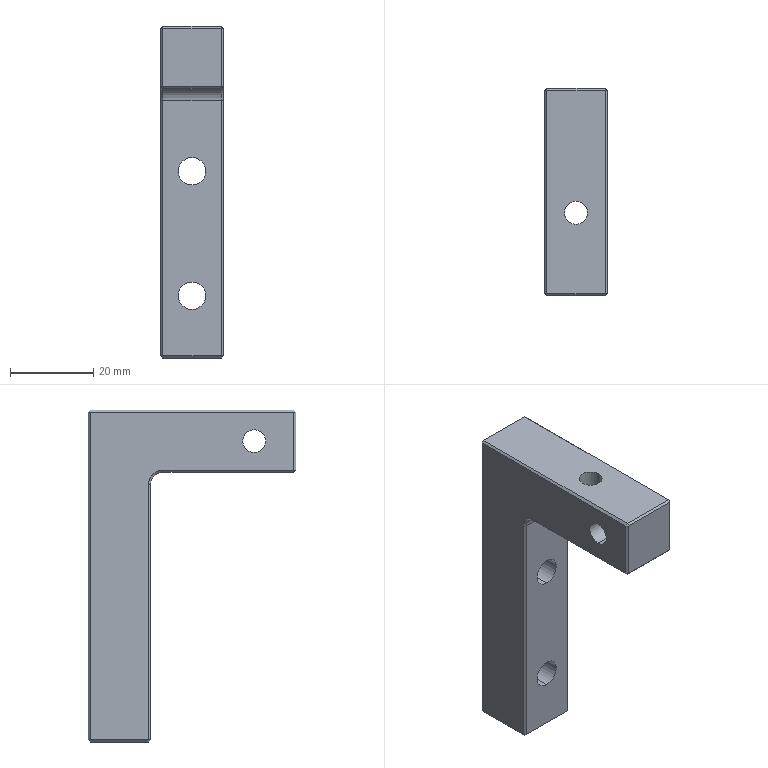Part | SolidWorks | features HoleWzd 3, Chamfer 1, Extrusion 1, Fillet 1, ICE 1, LPattern 1 | 1 solid | 46 faces | box 15 x 50 x 80 mm | volume 24092 mm3 | plane 35 | cylinder 9 | cone 2 | commonest cylinder face diameters 5.5 x4 6.6 x4 6 x1
STEP:
#1=CARTESIAN_POINT('',(97.5,-49.,204.8));
#2=VERTEX_POINT('',#1);
#3=CARTESIAN_POINT('',(97.5,-49.,198.2));
#4=VERTEX_POINT('',#3);
#5=CARTESIAN_POINT('',(97.5,-49.,201.5));
#6=DIRECTION('',(0.,-1.,0.));
#7=DIRECTION('',(0.,0.,-1.));
#8=AXIS2_PLACEMENT_3D('',#5,#6,#7);
#9=CIRCLE('',#8,3.3);
#10=EDGE_CURVE('',#2,#4,#9,.T.);
#11=ORIENTED_EDGE('',*,*,#10,.F.);
#12=CARTESIAN_POINT('',(97.5,-64.,204.8));
#13=VERTEX_POINT('',#12);
#14=CARTESIAN_POINT('',(97.5,-64.,204.8));
#15=DIRECTION('',(0.,-1.,0.));
#16=VECTOR('',#15,1000.);
#17=LINE('',#14,#16);
#18=EDGE_CURVE('',#2,#13,#17,.T.);
#19=ORIENTED_EDGE('',*,*,#18,.T.);
#20=CARTESIAN_POINT('',(97.5,-64.,198.2));
#21=VERTEX_POINT('',#20);
#22=CARTESIAN_POINT('',(97.5,-64.,201.5));
#23=DIRECTION('',(0.,-1.,0.));
#24=DIRECTION('',(0.,0.,-1.));
#25=AXIS2_PLACEMENT_3D('',#22,#23,#24);
#26=CIRCLE('',#25,3.3);
#27=EDGE_CURVE('',#13,#21,#26,.T.);
#28=ORIENTED_EDGE('',*,*,#27,.T.);
#29=CARTESIAN_POINT('',(97.5,-64.,198.2));
#30=DIRECTION('',(0.,-1.,0.));
#31=VECTOR('',#30,1000.);
#32=LINE('',#29,#31);
#33=EDGE_CURVE('',#4,#21,#32,.T.);
#34=ORIENTED_EDGE('',*,*,#33,.F.);
#35=EDGE_LOOP('',(#11,#19,#28,#34));
#36=FACE_OUTER_BOUND('',#35,.T.);
#37=CARTESIAN_POINT('',(97.5,-64.,201.5));
#38=DIRECTION('',(0.,-1.,0.));
#39=DIRECTION('',(0.,0.,-1.));
#40=AXIS2_PLACEMENT_3D('',#37,#38,#39);
#41=CYLINDRICAL_SURFACE('',#40,3.3);
#42=ADVANCED_FACE('',(#36),#41,.F.);
#43=CARTESIAN_POINT('',(105.,-89.,226.25));
#44=VERTEX_POINT('',#43);
#45=CARTESIAN_POINT('',(105.,-89.,231.75));
#46=VERTEX_POINT('',#45);
#47=CARTESIAN_POINT('',(105.,-89.,229.));
#48=DIRECTION('',(-1.,0.,0.));
#49=DIRECTION('',(0.,0.,1.));
#50=AXIS2_PLACEMENT_3D('',#47,#48,#49);
#51=CIRCLE('',#50,2.75);
#52=EDGE_CURVE('',#44,#46,#51,.T.);
#53=ORIENTED_EDGE('',*,*,#52,.F.);
#54=CARTESIAN_POINT('',(90.,-89.,226.25));
#55=VERTEX_POINT('',#54);
#56=CARTESIAN_POINT('',(90.,-89.,226.25));
#57=DIRECTION('',(-1.,0.,0.));
#58=VECTOR('',#57,1000.);
#59=LINE('',#56,#58);
#60=EDGE_CURVE('',#44,#55,#59,.T.);
#61=ORIENTED_EDGE('',*,*,#60,.T.);
#62=CARTESIAN_POINT('',(90.,-89.,231.75));
#63=VERTEX_POINT('',#62);
#64=CARTESIAN_POINT('',(90.,-89.,229.));
#65=DIRECTION('',(-1.,0.,0.));
#66=DIRECTION('',(0.,0.,1.));
#67=AXIS2_PLACEMENT_3D('',#64,#65,#66);
#68=CIRCLE('',#67,2.75);
#69=EDGE_CURVE('',#55,#63,#68,.T.);
#70=ORIENTED_EDGE('',*,*,#69,.T.);
#71=CARTESIAN_POINT('',(90.,-89.,231.75));
#72=DIRECTION('',(-1.,0.,0.));
#73=VECTOR('',#72,1000.);
#74=LINE('',#71,#73);
#75=EDGE_CURVE('',#46,#63,#74,.T.);
#76=ORIENTED_EDGE('',*,*,#75,.F.);
#77=EDGE_LOOP('',(#53,#61,#70,#76));
#78=FACE_OUTER_BOUND('',#77,.T.);
#79=CARTESIAN_POINT('',(90.,-89.,229.));
#80=DIRECTION('',(-1.,0.,0.));
#81=DIRECTION('',(0.,0.,1.));
#82=AXIS2_PLACEMENT_3D('',#79,#80,#81);
#83=CYLINDRICAL_SURFACE('',#82,2.75);
#84=ADVANCED_FACE('',(#78),#83,.F.);
#85=CARTESIAN_POINT('',(100.25,-79.,236.5));
#86=VERTEX_POINT('',#85);
#87=CARTESIAN_POINT('',(94.75,-79.,236.5));
#88=VERTEX_POINT('',#87);
#89=CARTESIAN_POINT('',(97.5,-79.,236.5));
#90=DIRECTION('',(0.,0.,-1.));
#91=DIRECTION('',(-1.,0.,0.));
#92=AXIS2_PLACEMENT_3D('',#89,#90,#91);
#93=CIRCLE('',#92,2.75);
#94=EDGE_CURVE('',#86,#88,#93,.T.);
#95=ORIENTED_EDGE('',*,*,#94,.F.);
#96=CARTESIAN_POINT('',(100.25,-79.,221.5));
#97=VERTEX_POINT('',#96);
#98=CARTESIAN_POINT('',(100.25,-79.,221.5));
#99=DIRECTION('',(0.,0.,-1.));
#100=VECTOR('',#99,1000.);
#101=LINE('',#98,#100);
#102=EDGE_CURVE('',#86,#97,#101,.T.);
#103=ORIENTED_EDGE('',*,*,#102,.T.);
#104=CARTESIAN_POINT('',(94.75,-79.,221.5));
#105=VERTEX_POINT('',#104);
#106=CARTESIAN_POINT('',(97.5,-79.,221.5));
#107=DIRECTION('',(0.,0.,-1.));
#108=DIRECTION('',(-1.,0.,0.));
#109=AXIS2_PLACEMENT_3D('',#106,#107,#108);
#110=CIRCLE('',#109,2.75);
#111=EDGE_CURVE('',#97,#105,#110,.T.);
#112=ORIENTED_EDGE('',*,*,#111,.T.);
#113=CARTESIAN_POINT('',(94.75,-79.,221.5));
#114=DIRECTION('',(0.,0.,-1.));
#115=VECTOR('',#114,1000.);
#116=LINE('',#113,#115);
#117=EDGE_CURVE('',#88,#105,#116,.T.);
#118=ORIENTED_EDGE('',*,*,#117,.F.);
#119=EDGE_LOOP('',(#95,#103,#112,#118));
#120=FACE_OUTER_BOUND('',#119,.T.);
#121=CARTESIAN_POINT('',(97.5,-79.,221.5));
#122=DIRECTION('',(0.,0.,-1.));
#123=DIRECTION('',(-1.,0.,0.));
#124=AXIS2_PLACEMENT_3D('',#121,#122,#123);
#125=CYLINDRICAL_SURFACE('',#124,2.75);
#126=ADVANCED_FACE('',(#120),#125,.F.);
#127=CARTESIAN_POINT('',(97.5,-49.,174.8));
#128=VERTEX_POINT('',#127);
#129=CARTESIAN_POINT('',(97.5,-49.,168.2));
#130=VERTEX_POINT('',#129);
#131=CARTESIAN_POINT('',(97.5,-49.,171.5));
#132=DIRECTION('',(0.,-1.,0.));
#133=DIRECTION('',(0.,0.,-1.));
#134=AXIS2_PLACEMENT_3D('',#131,#132,#133);
#135=CIRCLE('',#134,3.3);
#136=EDGE_CURVE('',#128,#130,#135,.T.);
#137=ORIENTED_EDGE('',*,*,#136,.F.);
#138=CARTESIAN_POINT('',(97.5,-64.,174.8));
#139=VERTEX_POINT('',#138);
#140=CARTESIAN_POINT('',(97.5,-64.,174.8));
#141=DIRECTION('',(0.,-1.,0.));
#142=VECTOR('',#141,1000.);
#143=LINE('',#140,#142);
#144=EDGE_CURVE('',#128,#139,#143,.T.);
#145=ORIENTED_EDGE('',*,*,#144,.T.);
#146=CARTESIAN_POINT('',(97.5,-64.,168.2));
#147=VERTEX_POINT('',#146);
#148=CARTESIAN_POINT('',(97.5,-64.,171.5));
#149=DIRECTION('',(0.,-1.,0.));
#150=DIRECTION('',(0.,0.,-1.));
#151=AXIS2_PLACEMENT_3D('',#148,#149,#150);
#152=CIRCLE('',#151,3.3);
#153=EDGE_CURVE('',#139,#147,#152,.T.);
#154=ORIENTED_EDGE('',*,*,#153,.T.);
#155=CARTESIAN_POINT('',(97.5,-64.,168.2));
#156=DIRECTION('',(0.,-1.,0.));
#157=VECTOR('',#156,1000.);
#158=LINE('',#155,#157);
#159=EDGE_CURVE('',#130,#147,#158,.T.);
#160=ORIENTED_EDGE('',*,*,#159,.F.);
#161=EDGE_LOOP('',(#137,#145,#154,#160));
#162=FACE_OUTER_BOUND('',#161,.T.);
#163=CARTESIAN_POINT('',(97.5,-64.,171.5));
#164=DIRECTION('',(0.,-1.,0.));
#165=DIRECTION('',(0.,0.,-1.));
#166=AXIS2_PLACEMENT_3D('',#163,#164,#165);
#167=CYLINDRICAL_SURFACE('',#166,3.3);
#168=ADVANCED_FACE('',(#162),#167,.F.);
#169=CARTESIAN_POINT('',(97.5,-64.,201.5));
#170=DIRECTION('',(0.,-1.,0.));
#171=DIRECTION('',(0.,0.,-1.));
#172=AXIS2_PLACEMENT_3D('',#169,#170,#171);
#173=CIRCLE('',#172,3.3);
#174=EDGE_CURVE('',#21,#13,#173,.T.);
#175=ORIENTED_EDGE('',*,*,#174,.F.);
#176=ORIENTED_EDGE('',*,*,#27,.F.);
#177=EDGE_LOOP('',(#175,#176));
#178=FACE_BOUND('',#177,.T.);
#179=CARTESIAN_POINT('',(104.5,-64.,218.5));
#180=VERTEX_POINT('',#179);
#181=CARTESIAN_POINT('',(90.5,-64.,218.5));
#182=VERTEX_POINT('',#181);
#183=CARTESIAN_POINT('',(90.,-64.,218.5));
#184=DIRECTION('',(-1.,0.,0.));
#185=VECTOR('',#184,1000.);
#186=LINE('',#183,#185);
#187=EDGE_CURVE('',#180,#182,#186,.T.);
#188=ORIENTED_EDGE('',*,*,#187,.T.);
#189=CARTESIAN_POINT('',(90.5,-64.,157.));
#190=VERTEX_POINT('',#189);
#191=CARTESIAN_POINT('',(90.5,-64.,156.5));
#192=DIRECTION('',(0.,0.,-1.));
#193=VECTOR('',#192,1000.);
#194=LINE('',#191,#193);
#195=EDGE_CURVE('',#182,#190,#194,.T.);
#196=ORIENTED_EDGE('',*,*,#195,.T.);
#197=CARTESIAN_POINT('',(104.5,-64.,157.));
#198=VERTEX_POINT('',#197);
#199=CARTESIAN_POINT('',(105.,-64.,157.));
#200=DIRECTION('',(1.,0.,0.));
#201=VECTOR('',#200,1000.);
#202=LINE('',#199,#201);
#203=EDGE_CURVE('',#190,#198,#202,.T.);
#204=ORIENTED_EDGE('',*,*,#203,.T.);
#205=CARTESIAN_POINT('',(104.5,-64.,156.5));
#206=DIRECTION('',(0.,0.,1.));
#207=VECTOR('',#206,1000.);
#208=LINE('',#205,#207);
#209=EDGE_CURVE('',#198,#180,#208,.T.);
#210=ORIENTED_EDGE('',*,*,#209,.T.);
#211=EDGE_LOOP('',(#188,#196,#204,#210));
#212=FACE_OUTER_BOUND('',#211,.T.);
#213=CARTESIAN_POINT('',(97.5,-64.,171.5));
#214=DIRECTION('',(0.,-1.,0.));
#215=DIRECTION('',(0.,0.,-1.));
#216=AXIS2_PLACEMENT_3D('',#213,#214,#215);
#217=CIRCLE('',#216,3.3);
#218=EDGE_CURVE('',#147,#139,#217,.T.);
#219=ORIENTED_EDGE('',*,*,#218,.F.);
#220=ORIENTED_EDGE('',*,*,#153,.F.);
#221=EDGE_LOOP('',(#219,#220));
#222=FACE_BOUND('',#221,.T.);
#223=CARTESIAN_POINT('',(105.,-64.,156.5));
#224=DIRECTION('',(0.,1.,0.));
#225=DIRECTION('',(0.,0.,1.));
#226=AXIS2_PLACEMENT_3D('',#223,#224,#225);
#227=PLANE('',#226);
#228=ADVANCED_FACE('',(#178,#212,#222),#227,.F.);
#229=CARTESIAN_POINT('',(90.,-89.,229.));
#230=DIRECTION('',(-1.,0.,0.));
#231=DIRECTION('',(0.,0.,1.));
#232=AXIS2_PLACEMENT_3D('',#229,#230,#231);
#233=CIRCLE('',#232,2.75);
#234=EDGE_CURVE('',#63,#55,#233,.T.);
#235=ORIENTED_EDGE('',*,*,#234,.F.);
#236=ORIENTED_EDGE('',*,*,#69,.F.);
#237=EDGE_LOOP('',(#235,#236));
#238=FACE_BOUND('',#237,.T.);
#239=CARTESIAN_POINT('',(90.,-49.5,157.));
#240=VERTEX_POINT('',#239);
#241=CARTESIAN_POINT('',(90.,-63.5,157.));
#242=VERTEX_POINT('',#241);
#243=CARTESIAN_POINT('',(90.,-64.,157.));
#244=DIRECTION('',(0.,-1.,0.));
#245=VECTOR('',#244,1000.);
#246=LINE('',#243,#245);
#247=EDGE_CURVE('',#240,#242,#246,.T.);
#248=ORIENTED_EDGE('',*,*,#247,.T.);
#249=CARTESIAN_POINT('',(90.,-63.5,218.5));
#250=VERTEX_POINT('',#249);
#251=CARTESIAN_POINT('',(90.,-63.5,156.5));
#252=DIRECTION('',(0.,0.,1.));
#253=VECTOR('',#252,1000.);
#254=LINE('',#251,#253);
#255=EDGE_CURVE('',#242,#250,#254,.T.);
#256=ORIENTED_EDGE('',*,*,#255,.T.);
#257=CARTESIAN_POINT('',(90.,-67.,222.));
#258=VERTEX_POINT('',#257);
#259=CARTESIAN_POINT('',(90.,-67.,218.5));
#260=DIRECTION('',(1.,0.,0.));
#261=DIRECTION('',(0.,0.,-1.));
#262=AXIS2_PLACEMENT_3D('',#259,#260,#261);
#263=CIRCLE('',#262,3.5);
#264=EDGE_CURVE('',#250,#258,#263,.T.);
#265=ORIENTED_EDGE('',*,*,#264,.T.);
#266=CARTESIAN_POINT('',(90.,-98.5,222.));
#267=VERTEX_POINT('',#266);
#268=CARTESIAN_POINT('',(90.,-49.,222.));
#269=DIRECTION('',(0.,-1.,0.));
#270=VECTOR('',#269,1000.);
#271=LINE('',#268,#270);
#272=EDGE_CURVE('',#258,#267,#271,.T.);
#273=ORIENTED_EDGE('',*,*,#272,.T.);
#274=CARTESIAN_POINT('',(90.,-98.5,236.));
#275=VERTEX_POINT('',#274);
#276=CARTESIAN_POINT('',(90.,-98.5,156.5));
#277=DIRECTION('',(0.,0.,1.));
#278=VECTOR('',#277,1000.);
#279=LINE('',#276,#278);
#280=EDGE_CURVE('',#267,#275,#279,.T.);
#281=ORIENTED_EDGE('',*,*,#280,.T.);
#282=CARTESIAN_POINT('',(90.,-49.5,236.));
#283=VERTEX_POINT('',#282);
#284=CARTESIAN_POINT('',(90.,-49.,236.));
#285=DIRECTION('',(0.,1.,0.));
#286=VECTOR('',#285,1000.);
#287=LINE('',#284,#286);
#288=EDGE_CURVE('',#275,#283,#287,.T.);
#289=ORIENTED_EDGE('',*,*,#288,.T.);
#290=CARTESIAN_POINT('',(90.,-49.5,156.5));
#291=DIRECTION('',(0.,0.,-1.));
#292=VECTOR('',#291,1000.);
#293=LINE('',#290,#292);
#294=EDGE_CURVE('',#283,#240,#293,.T.);
#295=ORIENTED_EDGE('',*,*,#294,.T.);
#296=EDGE_LOOP('',(#248,#256,#265,#273,#281,#289,#295));
#297=FACE_OUTER_BOUND('',#296,.T.);
#298=CARTESIAN_POINT('',(90.,-49.,156.5));
#299=DIRECTION('',(1.,0.,0.));
#300=DIRECTION('',(0.,0.,-1.));
#301=AXIS2_PLACEMENT_3D('',#298,#299,#300);
#302=PLANE('',#301);
#303=ADVANCED_FACE('',(#238,#297),#302,.F.);
#304=CARTESIAN_POINT('',(97.5,-49.,201.5));
#305=DIRECTION('',(0.,-1.,0.));
#306=DIRECTION('',(0.,0.,-1.));
#307=AXIS2_PLACEMENT_3D('',#304,#305,#306);
#308=CIRCLE('',#307,3.3);
#309=EDGE_CURVE('',#4,#2,#308,.T.);
#310=ORIENTED_EDGE('',*,*,#309,.T.);
#311=ORIENTED_EDGE('',*,*,#10,.T.);
#312=EDGE_LOOP('',(#310,#311));
#313=FACE_BOUND('',#312,.T.);
#314=CARTESIAN_POINT('',(90.5,-49.,236.));
#315=VERTEX_POINT('',#314);
#316=CARTESIAN_POINT('',(104.5,-49.,236.));
#317=VERTEX_POINT('',#316);
#318=CARTESIAN_POINT('',(90.,-49.,236.));
#319=DIRECTION('',(1.,0.,0.));
#320=VECTOR('',#319,1000.);
#321=LINE('',#318,#320);
#322=EDGE_CURVE('',#315,#317,#321,.T.);
#323=ORIENTED_EDGE('',*,*,#322,.T.);
#324=CARTESIAN_POINT('',(104.5,-49.,157.));
#325=VERTEX_POINT('',#324);
#326=CARTESIAN_POINT('',(104.5,-49.,156.5));
#327=DIRECTION('',(0.,0.,-1.));
#328=VECTOR('',#327,1000.);
#329=LINE('',#326,#328);
#330=EDGE_CURVE('',#317,#325,#329,.T.);
#331=ORIENTED_EDGE('',*,*,#330,.T.);
#332=CARTESIAN_POINT('',(90.5,-49.,157.));
#333=VERTEX_POINT('',#332);
#334=CARTESIAN_POINT('',(90.,-49.,157.));
#335=DIRECTION('',(-1.,0.,0.));
#336=VECTOR('',#335,1000.);
#337=LINE('',#334,#336);
#338=EDGE_CURVE('',#325,#333,#337,.T.);
#339=ORIENTED_EDGE('',*,*,#338,.T.);
#340=CARTESIAN_POINT('',(90.5,-49.,156.5));
#341=DIRECTION('',(0.,0.,1.));
#342=VECTOR('',#341,1000.);
#343=LINE('',#340,#342);
#344=EDGE_CURVE('',#333,#315,#343,.T.);
#345=ORIENTED_EDGE('',*,*,#344,.T.);
#346=EDGE_LOOP('',(#323,#331,#339,#345));
#347=FACE_OUTER_BOUND('',#346,.T.);
#348=CARTESIAN_POINT('',(97.5,-49.,171.5));
#349=DIRECTION('',(0.,-1.,0.));
#350=DIRECTION('',(0.,0.,-1.));
#351=AXIS2_PLACEMENT_3D('',#348,#349,#350);
#352=CIRCLE('',#351,3.3);
#353=EDGE_CURVE('',#130,#128,#352,.T.);
#354=ORIENTED_EDGE('',*,*,#353,.T.);
#355=ORIENTED_EDGE('',*,*,#136,.T.);
#356=EDGE_LOOP('',(#354,#355));
#357=FACE_BOUND('',#356,.T.);
#358=CARTESIAN_POINT('',(90.,-49.,156.5));
#359=DIRECTION('',(0.,-1.,0.));
#360=DIRECTION('',(1.,0.,0.));
#361=AXIS2_PLACEMENT_3D('',#358,#359,#360);
#362=PLANE('',#361);
#363=ADVANCED_FACE('',(#313,#347,#357),#362,.F.);
#364=CARTESIAN_POINT('',(105.,-89.,229.));
#365=DIRECTION('',(-1.,0.,0.));
#366=DIRECTION('',(0.,0.,1.));
#367=AXIS2_PLACEMENT_3D('',#364,#365,#366);
#368=CIRCLE('',#367,2.75);
#369=EDGE_CURVE('',#46,#44,#368,.T.);
#370=ORIENTED_EDGE('',*,*,#369,.T.);
#371=ORIENTED_EDGE('',*,*,#52,.T.);
#372=EDGE_LOOP('',(#370,#371));
#373=FACE_BOUND('',#372,.T.);
#374=CARTESIAN_POINT('',(105.,-63.5,157.));
#375=VERTEX_POINT('',#374);
#376=CARTESIAN_POINT('',(105.,-49.5,157.));
#377=VERTEX_POINT('',#376);
#378=CARTESIAN_POINT('',(105.,-49.,157.));
#379=DIRECTION('',(0.,1.,0.));
#380=VECTOR('',#379,1000.);
#381=LINE('',#378,#380);
#382=EDGE_CURVE('',#375,#377,#381,.T.);
#383=ORIENTED_EDGE('',*,*,#382,.T.);
#384=CARTESIAN_POINT('',(105.,-49.5,236.));
#385=VERTEX_POINT('',#384);
#386=CARTESIAN_POINT('',(105.,-49.5,156.5));
#387=DIRECTION('',(0.,0.,1.));
#388=VECTOR('',#387,1000.);
#389=LINE('',#386,#388);
#390=EDGE_CURVE('',#377,#385,#389,.T.);
#391=ORIENTED_EDGE('',*,*,#390,.T.);
#392=CARTESIAN_POINT('',(105.,-98.5,236.));
#393=VERTEX_POINT('',#392);
#394=CARTESIAN_POINT('',(105.,-49.,236.));
#395=DIRECTION('',(0.,-1.,0.));
#396=VECTOR('',#395,1000.);
#397=LINE('',#394,#396);
#398=EDGE_CURVE('',#385,#393,#397,.T.);
#399=ORIENTED_EDGE('',*,*,#398,.T.);
#400=CARTESIAN_POINT('',(105.,-98.5,222.));
#401=VERTEX_POINT('',#400);
#402=CARTESIAN_POINT('',(105.,-98.5,156.5));
#403=DIRECTION('',(0.,0.,-1.));
#404=VECTOR('',#403,1000.);
#405=LINE('',#402,#404);
#406=EDGE_CURVE('',#393,#401,#405,.T.);
#407=ORIENTED_EDGE('',*,*,#406,.T.);
#408=CARTESIAN_POINT('',(105.,-67.,222.));
#409=VERTEX_POINT('',#408);
#410=CARTESIAN_POINT('',(105.,-49.,222.));
#411=DIRECTION('',(0.,1.,0.));
#412=VECTOR('',#411,1000.);
#413=LINE('',#410,#412);
#414=EDGE_CURVE('',#401,#409,#413,.T.);
#415=ORIENTED_EDGE('',*,*,#414,.T.);
#416=CARTESIAN_POINT('',(105.,-63.5,218.5));
#417=VERTEX_POINT('',#416);
#418=CARTESIAN_POINT('',(105.,-67.,218.5));
#419=DIRECTION('',(-1.,0.,0.));
#420=DIRECTION('',(0.,-1.,0.));
#421=AXIS2_PLACEMENT_3D('',#418,#419,#420);
#422=CIRCLE('',#421,3.5);
#423=EDGE_CURVE('',#409,#417,#422,.T.);
#424=ORIENTED_EDGE('',*,*,#423,.T.);
#425=CARTESIAN_POINT('',(105.,-63.5,156.5));
#426=DIRECTION('',(0.,0.,-1.));
#427=VECTOR('',#426,1000.);
#428=LINE('',#425,#427);
#429=EDGE_CURVE('',#417,#375,#428,.T.);
#430=ORIENTED_EDGE('',*,*,#429,.T.);
#431=EDGE_LOOP('',(#383,#391,#399,#407,#415,#424,#430));
#432=FACE_OUTER_BOUND('',#431,.T.);
#433=CARTESIAN_POINT('',(105.,-49.,156.5));
#434=DIRECTION('',(-1.,0.,0.));
#435=DIRECTION('',(0.,-1.,0.));
#436=AXIS2_PLACEMENT_3D('',#433,#434,#435);
#437=PLANE('',#436);
#438=ADVANCED_FACE('',(#373,#432),#437,.F.);
#439=CARTESIAN_POINT('',(90.5,-49.5,156.5));
#440=VERTEX_POINT('',#439);
#441=CARTESIAN_POINT('',(104.5,-49.5,156.5));
#442=VERTEX_POINT('',#441);
#443=CARTESIAN_POINT('',(105.,-49.5,156.5));
#444=DIRECTION('',(1.,0.,0.));
#445=VECTOR('',#444,1000.);
#446=LINE('',#443,#445);
#447=EDGE_CURVE('',#440,#442,#446,.T.);
#448=ORIENTED_EDGE('',*,*,#447,.T.);
#449=CARTESIAN_POINT('',(104.5,-63.5,156.5));
#450=VERTEX_POINT('',#449);
#451=CARTESIAN_POINT('',(104.5,-64.,156.5));
#452=DIRECTION('',(0.,-1.,0.));
#453=VECTOR('',#452,1000.);
#454=LINE('',#451,#453);
#455=EDGE_CURVE('',#442,#450,#454,.T.);
#456=ORIENTED_EDGE('',*,*,#455,.T.);
#457=CARTESIAN_POINT('',(90.5,-63.5,156.5));
#458=VERTEX_POINT('',#457);
#459=CARTESIAN_POINT('',(90.,-63.5,156.5));
#460=DIRECTION('',(-1.,0.,0.));
#461=VECTOR('',#460,1000.);
#462=LINE('',#459,#461);
#463=EDGE_CURVE('',#450,#458,#462,.T.);
#464=ORIENTED_EDGE('',*,*,#463,.T.);
#465=CARTESIAN_POINT('',(90.5,-49.,156.5));
#466=DIRECTION('',(0.,1.,0.));
#467=VECTOR('',#466,1000.);
#468=LINE('',#465,#467);
#469=EDGE_CURVE('',#458,#440,#468,.T.);
#470=ORIENTED_EDGE('',*,*,#469,.T.);
#471=EDGE_LOOP('',(#448,#456,#464,#470));
#472=FACE_OUTER_BOUND('',#471,.T.);
#473=CARTESIAN_POINT('',(90.,-64.,156.5));
#474=DIRECTION('',(0.,0.,-1.));
#475=DIRECTION('',(-1.,0.,0.));
#476=AXIS2_PLACEMENT_3D('',#473,#474,#475);
#477=PLANE('',#476);
#478=ADVANCED_FACE('',(#472),#477,.T.);
#479=CARTESIAN_POINT('',(97.5,-79.,236.5));
#480=DIRECTION('',(0.,0.,-1.));
#481=DIRECTION('',(-1.,0.,0.));
#482=AXIS2_PLACEMENT_3D('',#479,#480,#481);
#483=CIRCLE('',#482,2.75);
#484=EDGE_CURVE('',#88,#86,#483,.T.);
#485=ORIENTED_EDGE('',*,*,#484,.T.);
#486=ORIENTED_EDGE('',*,*,#94,.T.);
#487=EDGE_LOOP('',(#485,#486));
#488=FACE_BOUND('',#487,.T.);
#489=CARTESIAN_POINT('',(90.5,-98.5,236.5));
#490=VERTEX_POINT('',#489);
#491=CARTESIAN_POINT('',(104.5,-98.5,236.5));
#492=VERTEX_POINT('',#491);
#493=CARTESIAN_POINT('',(90.,-98.5,236.5));
#494=DIRECTION('',(1.,0.,0.));
#495=VECTOR('',#494,1000.);
#496=LINE('',#493,#495);
#497=EDGE_CURVE('',#490,#492,#496,.T.);
#498=ORIENTED_EDGE('',*,*,#497,.T.);
#499=CARTESIAN_POINT('',(104.5,-49.5,236.5));
#500=VERTEX_POINT('',#499);
#501=CARTESIAN_POINT('',(104.5,-64.,236.5));
#502=DIRECTION('',(0.,1.,0.));
#503=VECTOR('',#502,1000.);
#504=LINE('',#501,#503);
#505=EDGE_CURVE('',#492,#500,#504,.T.);
#506=ORIENTED_EDGE('',*,*,#505,.T.);
#507=CARTESIAN_POINT('',(90.5,-49.5,236.5));
#508=VERTEX_POINT('',#507);
#509=CARTESIAN_POINT('',(90.,-49.5,236.5));
#510=DIRECTION('',(-1.,0.,0.));
#511=VECTOR('',#510,1000.);
#512=LINE('',#509,#511);
#513=EDGE_CURVE('',#500,#508,#512,.T.);
#514=ORIENTED_EDGE('',*,*,#513,.T.);
#515=CARTESIAN_POINT('',(90.5,-64.,236.5));
#516=DIRECTION('',(0.,-1.,0.));
#517=VECTOR('',#516,1000.);
#518=LINE('',#515,#517);
#519=EDGE_CURVE('',#508,#490,#518,.T.);
#520=ORIENTED_EDGE('',*,*,#519,.T.);
#521=EDGE_LOOP('',(#498,#506,#514,#520));
#522=FACE_OUTER_BOUND('',#521,.T.);
#523=CARTESIAN_POINT('',(90.,-64.,236.5));
#524=DIRECTION('',(0.,0.,-1.));
#525=DIRECTION('',(-1.,0.,0.));
#526=AXIS2_PLACEMENT_3D('',#523,#524,#525);
#527=PLANE('',#526);
#528=ADVANCED_FACE('',(#488,#522),#527,.F.);
#529=ORIENTED_EDGE('',*,*,#144,.F.);
#530=ORIENTED_EDGE('',*,*,#353,.F.);
#531=ORIENTED_EDGE('',*,*,#159,.T.);
#532=ORIENTED_EDGE('',*,*,#218,.T.);
#533=EDGE_LOOP('',(#529,#530,#531,#532));
#534=FACE_OUTER_BOUND('',#533,.T.);
#535=CARTESIAN_POINT('',(97.5,-64.,171.5));
#536=DIRECTION('',(0.,-1.,0.));
#537=DIRECTION('',(0.,0.,-1.));
#538=AXIS2_PLACEMENT_3D('',#535,#536,#537);
#539=CYLINDRICAL_SURFACE('',#538,3.3);
#540=ADVANCED_FACE('',(#534),#539,.F.);
#541=CARTESIAN_POINT('',(97.5,-79.,221.5));
#542=DIRECTION('',(0.,0.,-1.));
#543=DIRECTION('',(-1.,0.,0.));
#544=AXIS2_PLACEMENT_3D('',#541,#542,#543);
#545=CIRCLE('',#544,2.75);
#546=EDGE_CURVE('',#105,#97,#545,.T.);
#547=ORIENTED_EDGE('',*,*,#546,.F.);
#548=ORIENTED_EDGE('',*,*,#111,.F.);
#549=EDGE_LOOP('',(#547,#548));
#550=FACE_BOUND('',#549,.T.);
#551=CARTESIAN_POINT('',(90.5,-67.,221.5));
#552=VERTEX_POINT('',#551);
#553=CARTESIAN_POINT('',(104.5,-67.,221.5));
#554=VERTEX_POINT('',#553);
#555=CARTESIAN_POINT('',(105.,-67.,221.5));
#556=DIRECTION('',(1.,0.,0.));
#557=VECTOR('',#556,1000.);
#558=LINE('',#555,#557);
#559=EDGE_CURVE('',#552,#554,#558,.T.);
#560=ORIENTED_EDGE('',*,*,#559,.T.);
#561=CARTESIAN_POINT('',(104.5,-98.5,221.5));
#562=VERTEX_POINT('',#561);
#563=CARTESIAN_POINT('',(104.5,-99.,221.5));
#564=DIRECTION('',(0.,-1.,0.));
#565=VECTOR('',#564,1000.);
#566=LINE('',#563,#565);
#567=EDGE_CURVE('',#554,#562,#566,.T.);
#568=ORIENTED_EDGE('',*,*,#567,.T.);
#569=CARTESIAN_POINT('',(90.5,-98.5,221.5));
#570=VERTEX_POINT('',#569);
#571=CARTESIAN_POINT('',(90.,-98.5,221.5));
#572=DIRECTION('',(-1.,0.,0.));
#573=VECTOR('',#572,1000.);
#574=LINE('',#571,#573);
#575=EDGE_CURVE('',#562,#570,#574,.T.);
#576=ORIENTED_EDGE('',*,*,#575,.T.);
#577=CARTESIAN_POINT('',(90.5,-99.,221.5));
#578=DIRECTION('',(0.,1.,0.));
#579=VECTOR('',#578,1000.);
#580=LINE('',#577,#579);
#581=EDGE_CURVE('',#570,#552,#580,.T.);
#582=ORIENTED_EDGE('',*,*,#581,.T.);
#583=EDGE_LOOP('',(#560,#568,#576,#582));
#584=FACE_OUTER_BOUND('',#583,.T.);
#585=CARTESIAN_POINT('',(90.,-99.,221.5));
#586=DIRECTION('',(0.,0.,1.));
#587=DIRECTION('',(1.,0.,0.));
#588=AXIS2_PLACEMENT_3D('',#585,#586,#587);
#589=PLANE('',#588);
#590=ADVANCED_FACE('',(#550,#584),#589,.F.);
#591=CARTESIAN_POINT('',(90.5,-99.,222.));
#592=VERTEX_POINT('',#591);
#593=CARTESIAN_POINT('',(104.5,-99.,222.));
#594=VERTEX_POINT('',#593);
#595=CARTESIAN_POINT('',(90.,-99.,222.));
#596=DIRECTION('',(1.,0.,0.));
#597=VECTOR('',#596,1000.);
#598=LINE('',#595,#597);
#599=EDGE_CURVE('',#592,#594,#598,.T.);
#600=ORIENTED_EDGE('',*,*,#599,.T.);
#601=CARTESIAN_POINT('',(104.5,-99.,236.));
#602=VERTEX_POINT('',#601);
#603=CARTESIAN_POINT('',(104.5,-99.,236.5));
#604=DIRECTION('',(0.,0.,1.));
#605=VECTOR('',#604,1000.);
#606=LINE('',#603,#605);
#607=EDGE_CURVE('',#594,#602,#606,.T.);
#608=ORIENTED_EDGE('',*,*,#607,.T.);
#609=CARTESIAN_POINT('',(90.5,-99.,236.));
#610=VERTEX_POINT('',#609);
#611=CARTESIAN_POINT('',(90.,-99.,236.));
#612=DIRECTION('',(-1.,0.,0.));
#613=VECTOR('',#612,1000.);
#614=LINE('',#611,#613);
#615=EDGE_CURVE('',#602,#610,#614,.T.);
#616=ORIENTED_EDGE('',*,*,#615,.T.);
#617=CARTESIAN_POINT('',(90.5,-99.,236.5));
#618=DIRECTION('',(0.,0.,-1.));
#619=VECTOR('',#618,1000.);
#620=LINE('',#617,#619);
#621=EDGE_CURVE('',#610,#592,#620,.T.);
#622=ORIENTED_EDGE('',*,*,#621,.T.);
#623=EDGE_LOOP('',(#600,#608,#616,#622));
#624=FACE_OUTER_BOUND('',#623,.T.);
#625=CARTESIAN_POINT('',(90.,-99.,236.5));
#626=DIRECTION('',(0.,1.,0.));
#627=DIRECTION('',(0.,0.,1.));
#628=AXIS2_PLACEMENT_3D('',#625,#626,#627);
#629=PLANE('',#628);
#630=ADVANCED_FACE('',(#624),#629,.F.);
#631=ORIENTED_EDGE('',*,*,#559,.F.);
#632=CARTESIAN_POINT('',(90.5,-67.,218.5));
#633=DIRECTION('',(-1.,0.,0.));
#634=DIRECTION('',(0.,0.,-1.));
#635=AXIS2_PLACEMENT_3D('',#632,#633,#634);
#636=CIRCLE('',#635,3.);
#637=EDGE_CURVE('',#552,#182,#636,.T.);
#638=ORIENTED_EDGE('',*,*,#637,.T.);
#639=ORIENTED_EDGE('',*,*,#187,.F.);
#640=CARTESIAN_POINT('',(104.5,-67.,218.5));
#641=DIRECTION('',(1.,0.,0.));
#642=DIRECTION('',(0.,0.,1.));
#643=AXIS2_PLACEMENT_3D('',#640,#641,#642);
#644=CIRCLE('',#643,3.);
#645=EDGE_CURVE('',#180,#554,#644,.T.);
#646=ORIENTED_EDGE('',*,*,#645,.T.);
#647=EDGE_LOOP('',(#631,#638,#639,#646));
#648=FACE_OUTER_BOUND('',#647,.T.);
#649=CARTESIAN_POINT('',(90.,-67.,218.5));
#650=DIRECTION('',(-1.,0.,0.));
#651=DIRECTION('',(0.,0.,1.));
#652=AXIS2_PLACEMENT_3D('',#649,#650,#651);
#653=CYLINDRICAL_SURFACE('',#652,3.);
#654=ADVANCED_FACE('',(#648),#653,.F.);
#655=CARTESIAN_POINT('',(105.,-49.5,236.));
#656=DIRECTION('',(0.7071,0.,-0.7071));
#657=VECTOR('',#656,1000.);
#658=LINE('',#655,#657);
#659=EDGE_CURVE('',#500,#385,#658,.T.);
#660=ORIENTED_EDGE('',*,*,#659,.F.);
#661=ORIENTED_EDGE('',*,*,#505,.F.);
#662=CARTESIAN_POINT('',(104.75,-98.5,236.25));
#663=DIRECTION('',(-0.7071,0.,0.7071));
#664=VECTOR('',#663,1000.);
#665=LINE('',#662,#664);
#666=EDGE_CURVE('',#393,#492,#665,.T.);
#667=ORIENTED_EDGE('',*,*,#666,.F.);
#668=ORIENTED_EDGE('',*,*,#398,.F.);
#669=EDGE_LOOP('',(#660,#661,#667,#668));
#670=FACE_OUTER_BOUND('',#669,.T.);
#671=CARTESIAN_POINT('',(105.,-49.,236.));
#672=DIRECTION('',(-0.7071,0.,-0.7071));
#673=DIRECTION('',(-0.7071,0.,0.7071));
#674=AXIS2_PLACEMENT_3D('',#671,#672,#673);
#675=PLANE('',#674);
#676=ADVANCED_FACE('',(#670),#675,.F.);
#677=CARTESIAN_POINT('',(104.5,-49.25,236.25));
#678=DIRECTION('',(0.,0.7071,-0.7071));
#679=VECTOR('',#678,1000.);
#680=LINE('',#677,#679);
#681=EDGE_CURVE('',#500,#317,#680,.T.);
#682=ORIENTED_EDGE('',*,*,#681,.F.);
#683=ORIENTED_EDGE('',*,*,#659,.T.);
#684=CARTESIAN_POINT('',(105.,-49.5,236.));
#685=DIRECTION('',(0.7071,-0.7071,0.));
#686=VECTOR('',#685,1000.);
#687=LINE('',#684,#686);
#688=EDGE_CURVE('',#317,#385,#687,.T.);
#689=ORIENTED_EDGE('',*,*,#688,.F.);
#690=EDGE_LOOP('',(#682,#683,#689));
#691=FACE_OUTER_BOUND('',#690,.T.);
#692=CARTESIAN_POINT('',(105.,-49.5,236.));
#693=DIRECTION('',(0.5774,0.5774,0.5774));
#694=DIRECTION('',(-0.7071,0.7071,0.));
#695=AXIS2_PLACEMENT_3D('',#692,#693,#694);
#696=PLANE('',#695);
#697=ADVANCED_FACE('',(#691),#696,.T.);
#698=CARTESIAN_POINT('',(104.5,-99.,236.));
#699=DIRECTION('',(-0.7071,-0.7071,0.));
#700=VECTOR('',#699,1000.);
#701=LINE('',#698,#700);
#702=EDGE_CURVE('',#393,#602,#701,.T.);
#703=ORIENTED_EDGE('',*,*,#702,.F.);
#704=ORIENTED_EDGE('',*,*,#666,.T.);
#705=CARTESIAN_POINT('',(104.5,-99.,236.));
#706=DIRECTION('',(0.,0.7071,0.7071));
#707=VECTOR('',#706,1000.);
#708=LINE('',#705,#707);
#709=EDGE_CURVE('',#602,#492,#708,.T.);
#710=ORIENTED_EDGE('',*,*,#709,.F.);
#711=EDGE_LOOP('',(#703,#704,#710));
#712=FACE_OUTER_BOUND('',#711,.T.);
#713=CARTESIAN_POINT('',(104.5,-99.,236.));
#714=DIRECTION('',(0.5774,-0.5774,0.5774));
#715=DIRECTION('',(0.7071,0.7071,0.));
#716=AXIS2_PLACEMENT_3D('',#713,#714,#715);
#717=PLANE('',#716);
#718=ADVANCED_FACE('',(#712),#717,.T.);
#719=ORIENTED_EDGE('',*,*,#688,.T.);
#720=ORIENTED_EDGE('',*,*,#390,.F.);
#721=CARTESIAN_POINT('',(104.5,-49.,157.));
#722=DIRECTION('',(0.7071,-0.7071,0.));
#723=VECTOR('',#722,1000.);
#724=LINE('',#721,#723);
#725=EDGE_CURVE('',#325,#377,#724,.T.);
#726=ORIENTED_EDGE('',*,*,#725,.F.);
#727=ORIENTED_EDGE('',*,*,#330,.F.);
#728=EDGE_LOOP('',(#719,#720,#726,#727));
#729=FACE_OUTER_BOUND('',#728,.T.);
#730=CARTESIAN_POINT('',(105.,-49.5,156.5));
#731=DIRECTION('',(-0.7071,-0.7071,0.));
#732=DIRECTION('',(0.7071,-0.7071,0.));
#733=AXIS2_PLACEMENT_3D('',#730,#731,#732);
#734=PLANE('',#733);
#735=ADVANCED_FACE('',(#729),#734,.F.);
#736=ORIENTED_EDGE('',*,*,#681,.T.);
#737=ORIENTED_EDGE('',*,*,#322,.F.);
#738=CARTESIAN_POINT('',(90.5,-49.,236.));
#739=DIRECTION('',(0.,0.7071,-0.7071));
#740=VECTOR('',#739,1000.);
#741=LINE('',#738,#740);
#742=EDGE_CURVE('',#508,#315,#741,.T.);
#743=ORIENTED_EDGE('',*,*,#742,.F.);
#744=ORIENTED_EDGE('',*,*,#513,.F.);
#745=EDGE_LOOP('',(#736,#737,#743,#744));
#746=FACE_OUTER_BOUND('',#745,.T.);
#747=CARTESIAN_POINT('',(90.,-49.,236.));
#748=DIRECTION('',(0.,-0.7071,-0.7071));
#749=DIRECTION('',(0.,0.7071,-0.7071));
#750=AXIS2_PLACEMENT_3D('',#747,#748,#749);
#751=PLANE('',#750);
#752=ADVANCED_FACE('',(#746),#751,.F.);
#753=CARTESIAN_POINT('',(90.,-98.5,236.));
#754=DIRECTION('',(-0.7071,0.,-0.7071));
#755=VECTOR('',#754,1000.);
#756=LINE('',#753,#755);
#757=EDGE_CURVE('',#490,#275,#756,.T.);
#758=ORIENTED_EDGE('',*,*,#757,.F.);
#759=ORIENTED_EDGE('',*,*,#519,.F.);
#760=CARTESIAN_POINT('',(90.25,-49.5,236.25));
#761=DIRECTION('',(0.7071,0.,0.7071));
#762=VECTOR('',#761,1000.);
#763=LINE('',#760,#762);
#764=EDGE_CURVE('',#283,#508,#763,.T.);
#765=ORIENTED_EDGE('',*,*,#764,.F.);
#766=ORIENTED_EDGE('',*,*,#288,.F.);
#767=EDGE_LOOP('',(#758,#759,#765,#766));
#768=FACE_OUTER_BOUND('',#767,.T.);
#769=CARTESIAN_POINT('',(90.,-49.,236.));
#770=DIRECTION('',(0.7071,0.,-0.7071));
#771=DIRECTION('',(-0.7071,0.,-0.7071));
#772=AXIS2_PLACEMENT_3D('',#769,#770,#771);
#773=PLANE('',#772);
#774=ADVANCED_FACE('',(#768),#773,.F.);
#775=ORIENTED_EDGE('',*,*,#709,.T.);
#776=ORIENTED_EDGE('',*,*,#497,.F.);
#777=CARTESIAN_POINT('',(90.5,-98.75,236.25));
#778=DIRECTION('',(0.,0.7071,0.7071));
#779=VECTOR('',#778,1000.);
#780=LINE('',#777,#779);
#781=EDGE_CURVE('',#610,#490,#780,.T.);
#782=ORIENTED_EDGE('',*,*,#781,.F.);
#783=ORIENTED_EDGE('',*,*,#615,.F.);
#784=EDGE_LOOP('',(#775,#776,#782,#783));
#785=FACE_OUTER_BOUND('',#784,.T.);
#786=CARTESIAN_POINT('',(90.,-99.,236.));
#787=DIRECTION('',(0.,0.7071,-0.7071));
#788=DIRECTION('',(0.,0.7071,0.7071));
#789=AXIS2_PLACEMENT_3D('',#786,#787,#788);
#790=PLANE('',#789);
#791=ADVANCED_FACE('',(#785),#790,.F.);
#792=ORIENTED_EDGE('',*,*,#702,.T.);
#793=ORIENTED_EDGE('',*,*,#607,.F.);
#794=CARTESIAN_POINT('',(104.75,-98.75,222.));
#795=DIRECTION('',(-0.7071,-0.7071,0.));
#796=VECTOR('',#795,1000.);
#797=LINE('',#794,#796);
#798=EDGE_CURVE('',#401,#594,#797,.T.);
#799=ORIENTED_EDGE('',*,*,#798,.F.);
#800=ORIENTED_EDGE('',*,*,#406,.F.);
#801=EDGE_LOOP('',(#792,#793,#799,#800));
#802=FACE_OUTER_BOUND('',#801,.T.);
#803=CARTESIAN_POINT('',(104.5,-99.,236.5));
#804=DIRECTION('',(-0.7071,0.7071,0.));
#805=DIRECTION('',(-0.7071,-0.7071,0.));
#806=AXIS2_PLACEMENT_3D('',#803,#804,#805);
#807=PLANE('',#806);
#808=ADVANCED_FACE('',(#802),#807,.F.);
#809=CARTESIAN_POINT('',(104.5,-98.5,221.5));
#810=DIRECTION('',(0.7071,0.,0.7071));
#811=VECTOR('',#810,1000.);
#812=LINE('',#809,#811);
#813=EDGE_CURVE('',#562,#401,#812,.T.);
#814=ORIENTED_EDGE('',*,*,#813,.F.);
#815=ORIENTED_EDGE('',*,*,#567,.F.);
#816=CARTESIAN_POINT('',(105.,-67.,222.));
#817=DIRECTION('',(-0.7071,0.,-0.7071));
#818=VECTOR('',#817,1000.);
#819=LINE('',#816,#818);
#820=EDGE_CURVE('',#409,#554,#819,.T.);
#821=ORIENTED_EDGE('',*,*,#820,.F.);
#822=ORIENTED_EDGE('',*,*,#414,.F.);
#823=EDGE_LOOP('',(#814,#815,#821,#822));
#824=FACE_OUTER_BOUND('',#823,.T.);
#825=CARTESIAN_POINT('',(105.,-49.,222.));
#826=DIRECTION('',(-0.7071,0.,0.7071));
#827=DIRECTION('',(0.7071,0.,0.7071));
#828=AXIS2_PLACEMENT_3D('',#825,#826,#827);
#829=PLANE('',#828);
#830=ADVANCED_FACE('',(#824),#829,.F.);
#831=ORIENTED_EDGE('',*,*,#820,.T.);
#832=ORIENTED_EDGE('',*,*,#645,.F.);
#833=CARTESIAN_POINT('',(105.,-63.5,218.5));
#834=DIRECTION('',(-0.7071,-0.7071,0.));
#835=VECTOR('',#834,1000.);
#836=LINE('',#833,#835);
#837=EDGE_CURVE('',#417,#180,#836,.T.);
#838=ORIENTED_EDGE('',*,*,#837,.F.);
#839=ORIENTED_EDGE('',*,*,#423,.F.);
#840=EDGE_LOOP('',(#831,#832,#838,#839));
#841=FACE_OUTER_BOUND('',#840,.T.);
#842=CARTESIAN_POINT('',(105.,-67.,218.5));
#843=DIRECTION('',(1.,0.,0.));
#844=DIRECTION('',(0.,0.,-1.));
#845=AXIS2_PLACEMENT_3D('',#842,#843,#844);
#846=CONICAL_SURFACE('',#845,3.5,0.7854);
#847=ADVANCED_FACE('',(#841),#846,.F.);
#848=CARTESIAN_POINT('',(104.5,-49.,157.));
#849=DIRECTION('',(0.,-0.7071,-0.7071));
#850=VECTOR('',#849,1000.);
#851=LINE('',#848,#850);
#852=EDGE_CURVE('',#325,#442,#851,.T.);
#853=ORIENTED_EDGE('',*,*,#852,.F.);
#854=ORIENTED_EDGE('',*,*,#725,.T.);
#855=CARTESIAN_POINT('',(104.75,-49.5,156.75));
#856=DIRECTION('',(0.7071,0.,0.7071));
#857=VECTOR('',#856,1000.);
#858=LINE('',#855,#857);
#859=EDGE_CURVE('',#442,#377,#858,.T.);
#860=ORIENTED_EDGE('',*,*,#859,.F.);
#861=EDGE_LOOP('',(#853,#854,#860));
#862=FACE_OUTER_BOUND('',#861,.T.);
#863=CARTESIAN_POINT('',(104.5,-49.,157.));
#864=DIRECTION('',(0.5774,0.5774,-0.5774));
#865=DIRECTION('',(0.,0.7071,0.7071));
#866=AXIS2_PLACEMENT_3D('',#863,#864,#865);
#867=PLANE('',#866);
#868=ADVANCED_FACE('',(#862),#867,.T.);
#869=ORIENTED_EDGE('',*,*,#764,.T.);
#870=ORIENTED_EDGE('',*,*,#742,.T.);
#871=CARTESIAN_POINT('',(90.5,-49.,236.));
#872=DIRECTION('',(0.7071,0.7071,0.));
#873=VECTOR('',#872,1000.);
#874=LINE('',#871,#873);
#875=EDGE_CURVE('',#283,#315,#874,.T.);
#876=ORIENTED_EDGE('',*,*,#875,.F.);
#877=EDGE_LOOP('',(#869,#870,#876));
#878=FACE_OUTER_BOUND('',#877,.T.);
#879=CARTESIAN_POINT('',(90.5,-49.,236.));
#880=DIRECTION('',(-0.5774,0.5774,0.5774));
#881=DIRECTION('',(-0.7071,-0.7071,0.));
#882=AXIS2_PLACEMENT_3D('',#879,#880,#881);
#883=PLANE('',#882);
#884=ADVANCED_FACE('',(#878),#883,.T.);
#885=ORIENTED_EDGE('',*,*,#781,.T.);
#886=ORIENTED_EDGE('',*,*,#757,.T.);
#887=CARTESIAN_POINT('',(90.,-98.5,236.));
#888=DIRECTION('',(-0.7071,0.7071,0.));
#889=VECTOR('',#888,1000.);
#890=LINE('',#887,#889);
#891=EDGE_CURVE('',#610,#275,#890,.T.);
#892=ORIENTED_EDGE('',*,*,#891,.F.);
#893=EDGE_LOOP('',(#885,#886,#892));
#894=FACE_OUTER_BOUND('',#893,.T.);
#895=CARTESIAN_POINT('',(90.,-98.5,236.));
#896=DIRECTION('',(-0.5774,-0.5774,0.5774));
#897=DIRECTION('',(0.7071,-0.7071,0.));
#898=AXIS2_PLACEMENT_3D('',#895,#896,#897);
#899=PLANE('',#898);
#900=ADVANCED_FACE('',(#894),#899,.T.);
#901=ORIENTED_EDGE('',*,*,#813,.T.);
#902=ORIENTED_EDGE('',*,*,#798,.T.);
#903=CARTESIAN_POINT('',(104.5,-98.5,221.5));
#904=DIRECTION('',(0.,-0.7071,0.7071));
#905=VECTOR('',#904,1000.);
#906=LINE('',#903,#905);
#907=EDGE_CURVE('',#562,#594,#906,.T.);
#908=ORIENTED_EDGE('',*,*,#907,.F.);
#909=EDGE_LOOP('',(#901,#902,#908));
#910=FACE_OUTER_BOUND('',#909,.T.);
#911=CARTESIAN_POINT('',(104.5,-98.5,221.5));
#912=DIRECTION('',(0.5774,-0.5774,-0.5774));
#913=DIRECTION('',(0.7071,0.7071,0.));
#914=AXIS2_PLACEMENT_3D('',#911,#912,#913);
#915=PLANE('',#914);
#916=ADVANCED_FACE('',(#910),#915,.T.);
#917=ORIENTED_EDGE('',*,*,#837,.T.);
#918=ORIENTED_EDGE('',*,*,#209,.F.);
#919=CARTESIAN_POINT('',(104.75,-63.75,157.));
#920=DIRECTION('',(-0.7071,-0.7071,0.));
#921=VECTOR('',#920,1000.);
#922=LINE('',#919,#921);
#923=EDGE_CURVE('',#375,#198,#922,.T.);
#924=ORIENTED_EDGE('',*,*,#923,.F.);
#925=ORIENTED_EDGE('',*,*,#429,.F.);
#926=EDGE_LOOP('',(#917,#918,#924,#925));
#927=FACE_OUTER_BOUND('',#926,.T.);
#928=CARTESIAN_POINT('',(104.5,-64.,156.5));
#929=DIRECTION('',(-0.7071,0.7071,0.));
#930=DIRECTION('',(-0.7071,-0.7071,0.));
#931=AXIS2_PLACEMENT_3D('',#928,#929,#930);
#932=PLANE('',#931);
#933=ADVANCED_FACE('',(#927),#932,.F.);
#934=ORIENTED_EDGE('',*,*,#859,.T.);
#935=ORIENTED_EDGE('',*,*,#382,.F.);
#936=CARTESIAN_POINT('',(104.5,-63.5,156.5));
#937=DIRECTION('',(0.7071,0.,0.7071));
#938=VECTOR('',#937,1000.);
#939=LINE('',#936,#938);
#940=EDGE_CURVE('',#450,#375,#939,.T.);
#941=ORIENTED_EDGE('',*,*,#940,.F.);
#942=ORIENTED_EDGE('',*,*,#455,.F.);
#943=EDGE_LOOP('',(#934,#935,#941,#942));
#944=FACE_OUTER_BOUND('',#943,.T.);
#945=CARTESIAN_POINT('',(104.5,-64.,156.5));
#946=DIRECTION('',(0.7071,0.,-0.7071));
#947=DIRECTION('',(-0.7071,0.,-0.7071));
#948=AXIS2_PLACEMENT_3D('',#945,#946,#947);
#949=PLANE('',#948);
#950=ADVANCED_FACE('',(#944),#949,.T.);
#951=ORIENTED_EDGE('',*,*,#852,.T.);
#952=ORIENTED_EDGE('',*,*,#447,.F.);
#953=CARTESIAN_POINT('',(90.5,-49.,157.));
#954=DIRECTION('',(0.,-0.7071,-0.7071));
#955=VECTOR('',#954,1000.);
#956=LINE('',#953,#955);
#957=EDGE_CURVE('',#333,#440,#956,.T.);
#958=ORIENTED_EDGE('',*,*,#957,.F.);
#959=ORIENTED_EDGE('',*,*,#338,.F.);
#960=EDGE_LOOP('',(#951,#952,#958,#959));
#961=FACE_OUTER_BOUND('',#960,.T.);
#962=CARTESIAN_POINT('',(90.,-49.5,156.5));
#963=DIRECTION('',(0.,0.7071,-0.7071));
#964=DIRECTION('',(0.,0.7071,0.7071));
#965=AXIS2_PLACEMENT_3D('',#962,#963,#964);
#966=PLANE('',#965);
#967=ADVANCED_FACE('',(#961),#966,.T.);
#968=ORIENTED_EDGE('',*,*,#875,.T.);
#969=ORIENTED_EDGE('',*,*,#344,.F.);
#970=CARTESIAN_POINT('',(90.5,-49.,157.));
#971=DIRECTION('',(0.7071,0.7071,0.));
#972=VECTOR('',#971,1000.);
#973=LINE('',#970,#972);
#974=EDGE_CURVE('',#240,#333,#973,.T.);
#975=ORIENTED_EDGE('',*,*,#974,.F.);
#976=ORIENTED_EDGE('',*,*,#294,.F.);
#977=EDGE_LOOP('',(#968,#969,#975,#976));
#978=FACE_OUTER_BOUND('',#977,.T.);
#979=CARTESIAN_POINT('',(90.5,-49.,156.5));
#980=DIRECTION('',(0.7071,-0.7071,0.));
#981=DIRECTION('',(0.7071,0.7071,0.));
#982=AXIS2_PLACEMENT_3D('',#979,#980,#981);
#983=PLANE('',#982);
#984=ADVANCED_FACE('',(#978),#983,.F.);
#985=ORIENTED_EDGE('',*,*,#891,.T.);
#986=ORIENTED_EDGE('',*,*,#280,.F.);
#987=CARTESIAN_POINT('',(90.25,-98.75,222.));
#988=DIRECTION('',(-0.7071,0.7071,0.));
#989=VECTOR('',#988,1000.);
#990=LINE('',#987,#989);
#991=EDGE_CURVE('',#592,#267,#990,.T.);
#992=ORIENTED_EDGE('',*,*,#991,.F.);
#993=ORIENTED_EDGE('',*,*,#621,.F.);
#994=EDGE_LOOP('',(#985,#986,#992,#993));
#995=FACE_OUTER_BOUND('',#994,.T.);
#996=CARTESIAN_POINT('',(90.5,-99.,236.5));
#997=DIRECTION('',(0.7071,0.7071,0.));
#998=DIRECTION('',(-0.7071,0.7071,0.));
#999=AXIS2_PLACEMENT_3D('',#996,#997,#998);
#1000=PLANE('',#999);
#1001=ADVANCED_FACE('',(#995),#1000,.F.);
#1002=ORIENTED_EDGE('',*,*,#907,.T.);
#1003=ORIENTED_EDGE('',*,*,#599,.F.);
#1004=CARTESIAN_POINT('',(90.5,-98.5,221.5));
#1005=DIRECTION('',(0.,-0.7071,0.7071));
#1006=VECTOR('',#1005,1000.);
#1007=LINE('',#1004,#1006);
#1008=EDGE_CURVE('',#570,#592,#1007,.T.);
#1009=ORIENTED_EDGE('',*,*,#1008,.F.);
#1010=ORIENTED_EDGE('',*,*,#575,.F.);
#1011=EDGE_LOOP('',(#1002,#1003,#1009,#1010));
#1012=FACE_OUTER_BOUND('',#1011,.T.);
#1013=CARTESIAN_POINT('',(90.,-99.,222.));
#1014=DIRECTION('',(0.,0.7071,0.7071));
#1015=DIRECTION('',(0.,-0.7071,0.7071));
#1016=AXIS2_PLACEMENT_3D('',#1013,#1014,#1015);
#1017=PLANE('',#1016);
#1018=ADVANCED_FACE('',(#1012),#1017,.F.);
#1019=ORIENTED_EDGE('',*,*,#940,.T.);
#1020=ORIENTED_EDGE('',*,*,#923,.T.);
#1021=CARTESIAN_POINT('',(104.5,-63.5,156.5));
#1022=DIRECTION('',(0.,-0.7071,0.7071));
#1023=VECTOR('',#1022,1000.);
#1024=LINE('',#1021,#1023);
#1025=EDGE_CURVE('',#450,#198,#1024,.T.);
#1026=ORIENTED_EDGE('',*,*,#1025,.F.);
#1027=EDGE_LOOP('',(#1019,#1020,#1026));
#1028=FACE_OUTER_BOUND('',#1027,.T.);
#1029=CARTESIAN_POINT('',(104.5,-63.5,156.5));
#1030=DIRECTION('',(0.5774,-0.5774,-0.5774));
#1031=DIRECTION('',(0.,0.7071,-0.7071));
#1032=AXIS2_PLACEMENT_3D('',#1029,#1030,#1031);
#1033=PLANE('',#1032);
#1034=ADVANCED_FACE('',(#1028),#1033,.T.);
#1035=ORIENTED_EDGE('',*,*,#974,.T.);
#1036=ORIENTED_EDGE('',*,*,#957,.T.);
#1037=CARTESIAN_POINT('',(90.25,-49.5,156.75));
#1038=DIRECTION('',(0.7071,0.,-0.7071));
#1039=VECTOR('',#1038,1000.);
#1040=LINE('',#1037,#1039);
#1041=EDGE_CURVE('',#240,#440,#1040,.T.);
#1042=ORIENTED_EDGE('',*,*,#1041,.F.);
#1043=EDGE_LOOP('',(#1035,#1036,#1042));
#1044=FACE_OUTER_BOUND('',#1043,.T.);
#1045=CARTESIAN_POINT('',(90.5,-49.,157.));
#1046=DIRECTION('',(-0.5774,0.5774,-0.5774));
#1047=DIRECTION('',(0.,0.7071,0.7071));
#1048=AXIS2_PLACEMENT_3D('',#1045,#1046,#1047);
#1049=PLANE('',#1048);
#1050=ADVANCED_FACE('',(#1044),#1049,.T.);
#1051=ORIENTED_EDGE('',*,*,#1008,.T.);
#1052=ORIENTED_EDGE('',*,*,#991,.T.);
#1053=CARTESIAN_POINT('',(90.5,-98.5,221.5));
#1054=DIRECTION('',(-0.7071,0.,0.7071));
#1055=VECTOR('',#1054,1000.);
#1056=LINE('',#1053,#1055);
#1057=EDGE_CURVE('',#570,#267,#1056,.T.);
#1058=ORIENTED_EDGE('',*,*,#1057,.F.);
#1059=EDGE_LOOP('',(#1051,#1052,#1058));
#1060=FACE_OUTER_BOUND('',#1059,.T.);
#1061=CARTESIAN_POINT('',(90.5,-98.5,221.5));
#1062=DIRECTION('',(-0.5774,-0.5774,-0.5774));
#1063=DIRECTION('',(0.,0.7071,-0.7071));
#1064=AXIS2_PLACEMENT_3D('',#1061,#1062,#1063);
#1065=PLANE('',#1064);
#1066=ADVANCED_FACE('',(#1060),#1065,.T.);
#1067=ORIENTED_EDGE('',*,*,#1025,.T.);
#1068=ORIENTED_EDGE('',*,*,#203,.F.);
#1069=CARTESIAN_POINT('',(90.5,-64.,157.));
#1070=DIRECTION('',(0.,-0.7071,0.7071));
#1071=VECTOR('',#1070,1000.);
#1072=LINE('',#1069,#1071);
#1073=EDGE_CURVE('',#458,#190,#1072,.T.);
#1074=ORIENTED_EDGE('',*,*,#1073,.F.);
#1075=ORIENTED_EDGE('',*,*,#463,.F.);
#1076=EDGE_LOOP('',(#1067,#1068,#1074,#1075));
#1077=FACE_OUTER_BOUND('',#1076,.T.);
#1078=CARTESIAN_POINT('',(90.,-63.5,156.5));
#1079=DIRECTION('',(0.,-0.7071,-0.7071));
#1080=DIRECTION('',(0.,0.7071,-0.7071));
#1081=AXIS2_PLACEMENT_3D('',#1078,#1079,#1080);
#1082=PLANE('',#1081);
#1083=ADVANCED_FACE('',(#1077),#1082,.T.);
#1084=ORIENTED_EDGE('',*,*,#1041,.T.);
#1085=ORIENTED_EDGE('',*,*,#469,.F.);
#1086=CARTESIAN_POINT('',(90.25,-63.5,156.75));
#1087=DIRECTION('',(0.7071,0.,-0.7071));
#1088=VECTOR('',#1087,1000.);
#1089=LINE('',#1086,#1088);
#1090=EDGE_CURVE('',#242,#458,#1089,.T.);
#1091=ORIENTED_EDGE('',*,*,#1090,.F.);
#1092=ORIENTED_EDGE('',*,*,#247,.F.);
#1093=EDGE_LOOP('',(#1084,#1085,#1091,#1092));
#1094=FACE_OUTER_BOUND('',#1093,.T.);
#1095=CARTESIAN_POINT('',(90.5,-64.,156.5));
#1096=DIRECTION('',(-0.7071,0.,-0.7071));
#1097=DIRECTION('',(-0.7071,0.,0.7071));
#1098=AXIS2_PLACEMENT_3D('',#1095,#1096,#1097);
#1099=PLANE('',#1098);
#1100=ADVANCED_FACE('',(#1094),#1099,.T.);
#1101=ORIENTED_EDGE('',*,*,#1057,.T.);
#1102=ORIENTED_EDGE('',*,*,#272,.F.);
#1103=CARTESIAN_POINT('',(90.5,-67.,221.5));
#1104=DIRECTION('',(-0.7071,0.,0.7071));
#1105=VECTOR('',#1104,1000.);
#1106=LINE('',#1103,#1105);
#1107=EDGE_CURVE('',#552,#258,#1106,.T.);
#1108=ORIENTED_EDGE('',*,*,#1107,.F.);
#1109=ORIENTED_EDGE('',*,*,#581,.F.);
#1110=EDGE_LOOP('',(#1101,#1102,#1108,#1109));
#1111=FACE_OUTER_BOUND('',#1110,.T.);
#1112=CARTESIAN_POINT('',(90.5,-99.,221.5));
#1113=DIRECTION('',(0.7071,0.,0.7071));
#1114=DIRECTION('',(0.7071,0.,-0.7071));
#1115=AXIS2_PLACEMENT_3D('',#1112,#1113,#1114);
#1116=PLANE('',#1115);
#1117=ADVANCED_FACE('',(#1111),#1116,.F.);
#1118=ORIENTED_EDGE('',*,*,#1090,.T.);
#1119=ORIENTED_EDGE('',*,*,#1073,.T.);
#1120=CARTESIAN_POINT('',(90.5,-64.,157.));
#1121=DIRECTION('',(0.7071,-0.7071,0.));
#1122=VECTOR('',#1121,1000.);
#1123=LINE('',#1120,#1122);
#1124=EDGE_CURVE('',#242,#190,#1123,.T.);
#1125=ORIENTED_EDGE('',*,*,#1124,.F.);
#1126=EDGE_LOOP('',(#1118,#1119,#1125));
#1127=FACE_OUTER_BOUND('',#1126,.T.);
#1128=CARTESIAN_POINT('',(90.5,-64.,157.));
#1129=DIRECTION('',(-0.5774,-0.5774,-0.5774));
#1130=DIRECTION('',(0.,0.7071,-0.7071));
#1131=AXIS2_PLACEMENT_3D('',#1128,#1129,#1130);
#1132=PLANE('',#1131);
#1133=ADVANCED_FACE('',(#1127),#1132,.T.);
#1134=ORIENTED_EDGE('',*,*,#1107,.T.);
#1135=ORIENTED_EDGE('',*,*,#264,.F.);
#1136=CARTESIAN_POINT('',(90.5,-64.,218.5));
#1137=DIRECTION('',(-0.7071,0.7071,0.));
#1138=VECTOR('',#1137,1000.);
#1139=LINE('',#1136,#1138);
#1140=EDGE_CURVE('',#182,#250,#1139,.T.);
#1141=ORIENTED_EDGE('',*,*,#1140,.F.);
#1142=ORIENTED_EDGE('',*,*,#637,.F.);
#1143=EDGE_LOOP('',(#1134,#1135,#1141,#1142));
#1144=FACE_OUTER_BOUND('',#1143,.T.);
#1145=CARTESIAN_POINT('',(90.,-67.,218.5));
#1146=DIRECTION('',(-1.,0.,0.));
#1147=DIRECTION('',(0.,0.,1.));
#1148=AXIS2_PLACEMENT_3D('',#1145,#1146,#1147);
#1149=CONICAL_SURFACE('',#1148,3.5,0.7854);
#1150=ADVANCED_FACE('',(#1144),#1149,.F.);
#1151=ORIENTED_EDGE('',*,*,#1124,.T.);
#1152=ORIENTED_EDGE('',*,*,#195,.F.);
#1153=ORIENTED_EDGE('',*,*,#1140,.T.);
#1154=ORIENTED_EDGE('',*,*,#255,.F.);
#1155=EDGE_LOOP('',(#1151,#1152,#1153,#1154));
#1156=FACE_OUTER_BOUND('',#1155,.T.);
#1157=CARTESIAN_POINT('',(90.,-63.5,156.5));
#1158=DIRECTION('',(0.7071,0.7071,0.));
#1159=DIRECTION('',(-0.7071,0.7071,0.));
#1160=AXIS2_PLACEMENT_3D('',#1157,#1158,#1159);
#1161=PLANE('',#1160);
#1162=ADVANCED_FACE('',(#1156),#1161,.F.);
#1163=ORIENTED_EDGE('',*,*,#102,.F.);
#1164=ORIENTED_EDGE('',*,*,#484,.F.);
#1165=ORIENTED_EDGE('',*,*,#117,.T.);
#1166=ORIENTED_EDGE('',*,*,#546,.T.);
#1167=EDGE_LOOP('',(#1163,#1164,#1165,#1166));
#1168=FACE_OUTER_BOUND('',#1167,.T.);
#1169=CARTESIAN_POINT('',(97.5,-79.,221.5));
#1170=DIRECTION('',(0.,0.,-1.));
#1171=DIRECTION('',(-1.,0.,0.));
#1172=AXIS2_PLACEMENT_3D('',#1169,#1170,#1171);
#1173=CYLINDRICAL_SURFACE('',#1172,2.75);
#1174=ADVANCED_FACE('',(#1168),#1173,.F.);
#1175=ORIENTED_EDGE('',*,*,#60,.F.);
#1176=ORIENTED_EDGE('',*,*,#369,.F.);
#1177=ORIENTED_EDGE('',*,*,#75,.T.);
#1178=ORIENTED_EDGE('',*,*,#234,.T.);
#1179=EDGE_LOOP('',(#1175,#1176,#1177,#1178));
#1180=FACE_OUTER_BOUND('',#1179,.T.);
#1181=CARTESIAN_POINT('',(90.,-89.,229.));
#1182=DIRECTION('',(-1.,0.,0.));
#1183=DIRECTION('',(0.,0.,1.));
#1184=AXIS2_PLACEMENT_3D('',#1181,#1182,#1183);
#1185=CYLINDRICAL_SURFACE('',#1184,2.75);
#1186=ADVANCED_FACE('',(#1180),#1185,.F.);
#1187=ORIENTED_EDGE('',*,*,#18,.F.);
#1188=ORIENTED_EDGE('',*,*,#309,.F.);
#1189=ORIENTED_EDGE('',*,*,#33,.T.);
#1190=ORIENTED_EDGE('',*,*,#174,.T.);
#1191=EDGE_LOOP('',(#1187,#1188,#1189,#1190));
#1192=FACE_OUTER_BOUND('',#1191,.T.);
#1193=CARTESIAN_POINT('',(97.5,-64.,201.5));
#1194=DIRECTION('',(0.,-1.,0.));
#1195=DIRECTION('',(0.,0.,-1.));
#1196=AXIS2_PLACEMENT_3D('',#1193,#1194,#1195);
#1197=CYLINDRICAL_SURFACE('',#1196,3.3);
#1198=ADVANCED_FACE('',(#1192),#1197,.F.);
#1199=CLOSED_SHELL('',(#42,#84,#126,#168,#228,#303,#363,#438,#478,#528,#540,#590,#630,#654,#676,#697,#718,#735,#752,#774,#791,#808,#830,#847,#868,#884,#900,#916,#933,#950,#967,#984,#1001,#1018,#1034,#1050,#1066,#1083,#1100,#1117,#1133,#1150,#1162,#1174,#1186,#1198));
#1200=MANIFOLD_SOLID_BREP('',#1199);
#1201=CARTESIAN_POINT('',(0.,0.,0.));
#1202=DIRECTION('',(0.,0.,1.));
#1203=DIRECTION('',(1.,0.,0.));
#1204=AXIS2_PLACEMENT_3D('',#1201,#1202,#1203);
#1205=(LENGTH_UNIT()NAMED_UNIT(*)SI_UNIT(.MILLI.,.METRE.));
#1206=UNCERTAINTY_MEASURE_WITH_UNIT(LENGTH_MEASURE(0.00001),#1205,'','');
#1207=(NAMED_UNIT(*)PLANE_ANGLE_UNIT()SI_UNIT($,.RADIAN.));
#1208=(NAMED_UNIT(*)SI_UNIT($,.STERADIAN.)SOLID_ANGLE_UNIT());
#1209=(GEOMETRIC_REPRESENTATION_CONTEXT(3)GLOBAL_UNCERTAINTY_ASSIGNED_CONTEXT((#1206))GLOBAL_UNIT_ASSIGNED_CONTEXT((#1205,#1207,#1208))REPRESENTATION_CONTEXT('',''));
#1210=ADVANCED_BREP_SHAPE_REPRESENTATION('',(#1200,#1204),#1209);